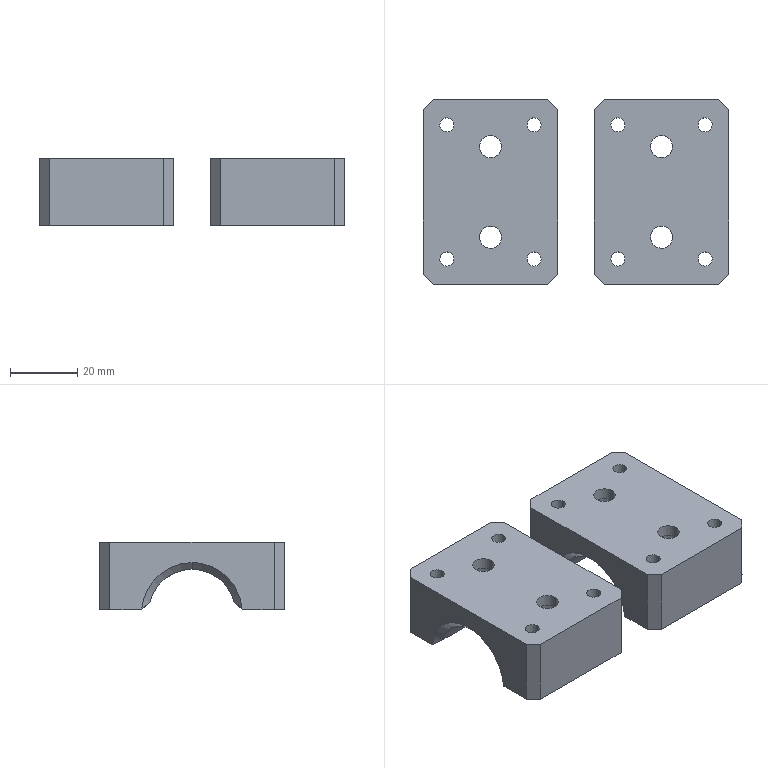NC program | NX | posted with a generic post | part box 91 x 55 x 20 mm
Lines 1 to 72 of 95737:
N10 G17 G21 G94 G90
(FLOOR_WALL_COPY , TOOL : D80)
N12 T19 M6
N14 G54
N16 G17 G0 G90 X-92.5 Y0. S6500 M3
N18 G43 Z30. H19
N20 Z3.
N22 G94 G1 Z0. F1500.
N24 X-87.5
N26 X87.5
N28 X92.5
N30 Z3.
N32 G0 Z30.
N34 M5
(DRILLING_COPY_1 , TOOL : D6A45)
N36 T01 M6
N38 G54
N40 G17 G0 G90 X-38.5 Y-20. S5000 M3
N42 G43 Z30. H1
N44 G94 G81 G98 Z-2.2 F350. R3.
N46 X-25.5 Y-13.5
N48 X-12.5 Y-20.
N50 X12.5
N52 X25.5 Y-13.5
N54 X38.5 Y-20.
N56 Y20.
N58 X25.5 Y13.5
N60 X12.5 Y20.
N62 X-12.5
N64 X-25.5 Y13.5
N66 X-38.5 Y20.
N68 G80
N70 G0 X-38.5 Y20. Z30.
N72 M5
(DRILLING_COPY_COPY , TOOL : 4.2ZT)
N74 T04 M6
N76 G54
N78 G17 G0 G90 X-38.5 Y-20. S2000 M3
N80 G43 Z30. H4
N82 G94 G83 G98 Z-22.762 F180. Q2. R3.
N84 X-12.5
N86 X12.5
N88 X38.5
N90 Y20.
N92 X12.5
N94 X-12.5
N96 X-38.5
N98 G80
N100 G0 X-38.5 Y20. Z30.
N102 M5
(DRILLING_COPY_COPY_COPY , TOOL : 6.6ZT)
N104 T16 M6
N106 G54
N108 G17 G0 G90 X-25.5 Y13.5 S2000 M3
N110 G43 Z30. H16
N112 G94 G83 G98 Z-23.483 F180. Q2. R3.
N114 Y-13.5
N116 X25.5
N118 Y13.5
N120 G80
N122 G0 X25.5 Y13.5 Z30.
N124 M5